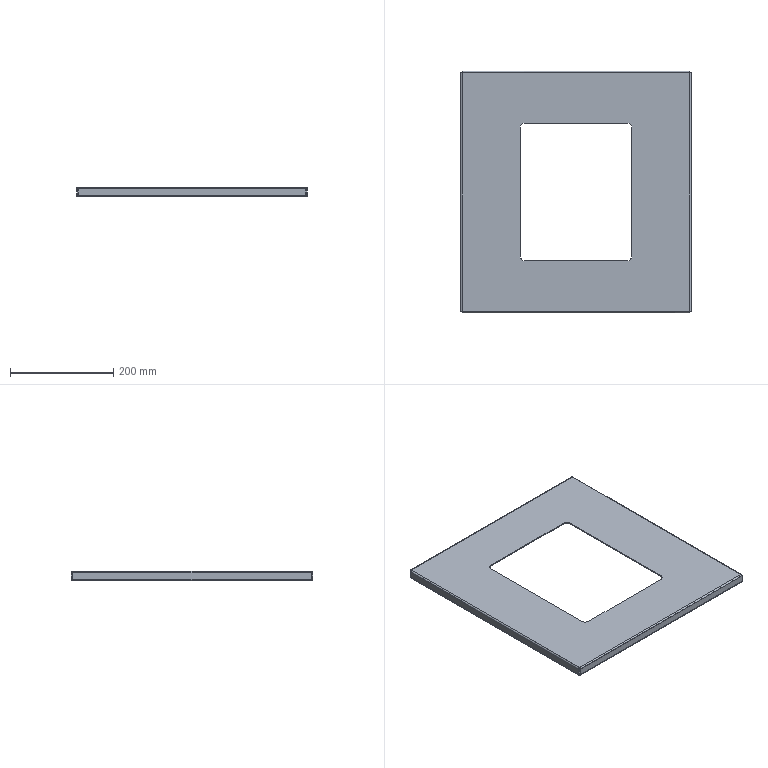Part | STEP file | MYT-A01-P24 | 1 solid | 78 faces | box 448 x 469 x 18 mm | volume 435629 mm3 | plane 42 | cylinder 20 | spline 16 | commonest cylinder face diameters 1.473 x8 5.473 x8 20 x4